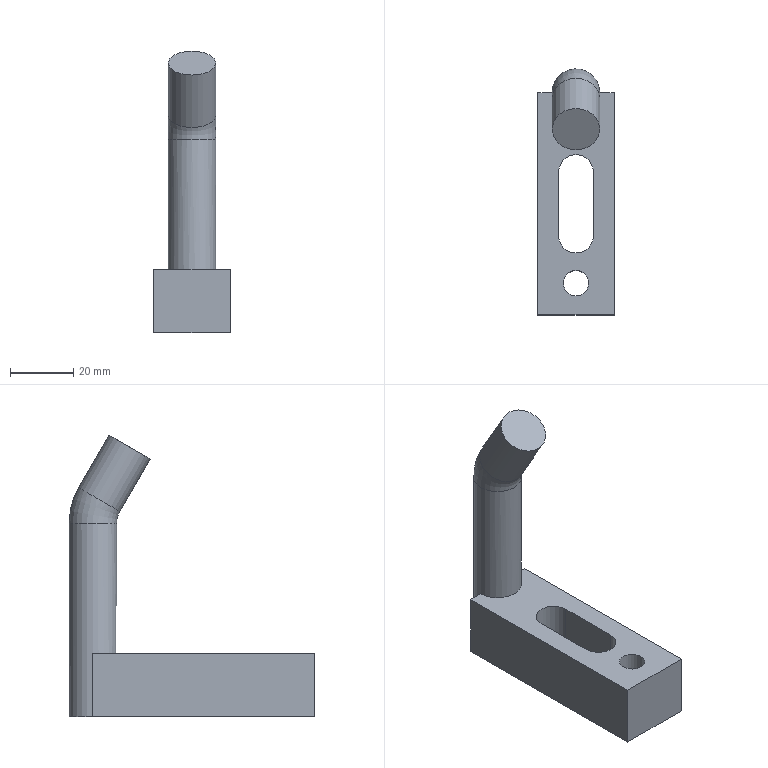Part | NX | features solid 2 | 1 solid | 16 faces | box 24 x 77.5 x 88.75 mm | volume 40062 mm3 | plane 10 | cylinder 5 | torus 1 | commonest cylinder face diameters 11 x2 15 x2 8 x1
STEP:
#1=CARTESIAN_POINT('',(67.5,315.,-15.));
#2=VERTEX_POINT('',#1);
#3=CARTESIAN_POINT('',(63.,315.,-15.));
#4=VERTEX_POINT('',#3);
#5=CARTESIAN_POINT('',(87.,315.,-15.));
#6=DIRECTION('',(-1.,0.,0.));
#7=VECTOR('',#6,1000.);
#8=LINE('',#5,#7);
#9=EDGE_CURVE('',#2,#4,#8,.T.);
#10=ORIENTED_EDGE('',*,*,#9,.F.);
#11=CARTESIAN_POINT('',(82.5,315.,-15.));
#12=VERTEX_POINT('',#11);
#13=CARTESIAN_POINT('',(75.,315.,-15.));
#14=DIRECTION('',(0.,0.,1.));
#15=DIRECTION('',(0.,-1.,0.));
#16=AXIS2_PLACEMENT_3D('',#13,#14,#15);
#17=CIRCLE('',#16,7.5);
#18=EDGE_CURVE('',#12,#2,#17,.T.);
#19=ORIENTED_EDGE('',*,*,#18,.F.);
#20=CARTESIAN_POINT('',(87.,315.,-15.));
#21=VERTEX_POINT('',#20);
#22=CARTESIAN_POINT('',(87.,315.,-15.));
#23=DIRECTION('',(-1.,0.,0.));
#24=VECTOR('',#23,1000.);
#25=LINE('',#22,#24);
#26=EDGE_CURVE('',#21,#12,#25,.T.);
#27=ORIENTED_EDGE('',*,*,#26,.F.);
#28=CARTESIAN_POINT('',(87.,245.,-15.));
#29=VERTEX_POINT('',#28);
#30=CARTESIAN_POINT('',(87.,245.,-15.));
#31=DIRECTION('',(0.,1.,0.));
#32=VECTOR('',#31,1000.);
#33=LINE('',#30,#32);
#34=EDGE_CURVE('',#29,#21,#33,.T.);
#35=ORIENTED_EDGE('',*,*,#34,.F.);
#36=CARTESIAN_POINT('',(63.,245.,-15.));
#37=VERTEX_POINT('',#36);
#38=CARTESIAN_POINT('',(63.,245.,-15.));
#39=DIRECTION('',(1.,0.,0.));
#40=VECTOR('',#39,1000.);
#41=LINE('',#38,#40);
#42=EDGE_CURVE('',#37,#29,#41,.T.);
#43=ORIENTED_EDGE('',*,*,#42,.F.);
#44=CARTESIAN_POINT('',(63.,315.,-15.));
#45=DIRECTION('',(0.,-1.,0.));
#46=VECTOR('',#45,1000.);
#47=LINE('',#44,#46);
#48=EDGE_CURVE('',#4,#37,#47,.T.);
#49=ORIENTED_EDGE('',*,*,#48,.F.);
#50=EDGE_LOOP('',(#10,#19,#27,#35,#43,#49));
#51=FACE_BOUND('',#50,.T.);
#52=CARTESIAN_POINT('',(69.5,270.,-15.));
#53=VERTEX_POINT('',#52);
#54=CARTESIAN_POINT('',(80.5,270.,-15.));
#55=VERTEX_POINT('',#54);
#56=CARTESIAN_POINT('',(75.,270.,-15.));
#57=DIRECTION('',(0.,0.,1.));
#58=DIRECTION('',(0.,-1.,0.));
#59=AXIS2_PLACEMENT_3D('',#56,#57,#58);
#60=CIRCLE('',#59,5.5);
#61=EDGE_CURVE('',#53,#55,#60,.T.);
#62=ORIENTED_EDGE('',*,*,#61,.T.);
#63=CARTESIAN_POINT('',(80.5,290.,-15.));
#64=VERTEX_POINT('',#63);
#65=CARTESIAN_POINT('',(80.5,290.,-15.));
#66=DIRECTION('',(0.,-1.,0.));
#67=VECTOR('',#66,1000.);
#68=LINE('',#65,#67);
#69=EDGE_CURVE('',#64,#55,#68,.T.);
#70=ORIENTED_EDGE('',*,*,#69,.F.);
#71=CARTESIAN_POINT('',(69.5,290.,-15.));
#72=VERTEX_POINT('',#71);
#73=CARTESIAN_POINT('',(75.,290.,-15.));
#74=DIRECTION('',(0.,0.,1.));
#75=DIRECTION('',(0.,-1.,0.));
#76=AXIS2_PLACEMENT_3D('',#73,#74,#75);
#77=CIRCLE('',#76,5.5);
#78=EDGE_CURVE('',#64,#72,#77,.T.);
#79=ORIENTED_EDGE('',*,*,#78,.T.);
#80=CARTESIAN_POINT('',(69.5,290.,-15.));
#81=DIRECTION('',(0.,-1.,0.));
#82=VECTOR('',#81,1000.);
#83=LINE('',#80,#82);
#84=EDGE_CURVE('',#72,#53,#83,.T.);
#85=ORIENTED_EDGE('',*,*,#84,.T.);
#86=EDGE_LOOP('',(#62,#70,#79,#85));
#87=FACE_BOUND('',#86,.T.);
#88=CARTESIAN_POINT('',(75.,251.,-15.));
#89=VERTEX_POINT('',#88);
#90=CARTESIAN_POINT('',(75.,255.,-15.));
#91=DIRECTION('',(0.,0.,1.));
#92=DIRECTION('',(0.,-1.,0.));
#93=AXIS2_PLACEMENT_3D('',#90,#91,#92);
#94=CIRCLE('',#93,4.);
#95=EDGE_CURVE('',#89,#89,#94,.T.);
#96=ORIENTED_EDGE('',*,*,#95,.T.);
#97=EDGE_LOOP('',(#96));
#98=FACE_BOUND('',#97,.T.);
#99=CARTESIAN_POINT('',(87.,245.,-15.));
#100=DIRECTION('',(0.,0.,1.));
#101=DIRECTION('',(0.,-1.,0.));
#102=AXIS2_PLACEMENT_3D('',#99,#100,#101);
#103=PLANE('',#102);
#104=ADVANCED_FACE('',(#51,#87,#98),#103,.F.);
#105=ORIENTED_EDGE('',*,*,#34,.T.);
#106=CARTESIAN_POINT('',(87.,315.,5.));
#107=VERTEX_POINT('',#106);
#108=CARTESIAN_POINT('',(87.,315.,5.));
#109=DIRECTION('',(0.,0.,-1.));
#110=VECTOR('',#109,1000.);
#111=LINE('',#108,#110);
#112=EDGE_CURVE('',#107,#21,#111,.T.);
#113=ORIENTED_EDGE('',*,*,#112,.F.);
#114=CARTESIAN_POINT('',(87.,245.,5.));
#115=VERTEX_POINT('',#114);
#116=CARTESIAN_POINT('',(87.,245.,5.));
#117=DIRECTION('',(0.,1.,0.));
#118=VECTOR('',#117,1000.);
#119=LINE('',#116,#118);
#120=EDGE_CURVE('',#115,#107,#119,.T.);
#121=ORIENTED_EDGE('',*,*,#120,.F.);
#122=CARTESIAN_POINT('',(87.,245.,5.));
#123=DIRECTION('',(0.,0.,-1.));
#124=VECTOR('',#123,1000.);
#125=LINE('',#122,#124);
#126=EDGE_CURVE('',#115,#29,#125,.T.);
#127=ORIENTED_EDGE('',*,*,#126,.T.);
#128=EDGE_LOOP('',(#105,#113,#121,#127));
#129=FACE_BOUND('',#128,.T.);
#130=CARTESIAN_POINT('',(87.,245.,5.));
#131=DIRECTION('',(-1.,0.,0.));
#132=DIRECTION('',(0.,-1.,0.));
#133=AXIS2_PLACEMENT_3D('',#130,#131,#132);
#134=PLANE('',#133);
#135=ADVANCED_FACE('',(#129),#134,.F.);
#136=ORIENTED_EDGE('',*,*,#42,.T.);
#137=ORIENTED_EDGE('',*,*,#126,.F.);
#138=CARTESIAN_POINT('',(63.,245.,5.));
#139=VERTEX_POINT('',#138);
#140=CARTESIAN_POINT('',(63.,245.,5.));
#141=DIRECTION('',(1.,0.,0.));
#142=VECTOR('',#141,1000.);
#143=LINE('',#140,#142);
#144=EDGE_CURVE('',#139,#115,#143,.T.);
#145=ORIENTED_EDGE('',*,*,#144,.F.);
#146=CARTESIAN_POINT('',(63.,245.,5.));
#147=DIRECTION('',(0.,0.,-1.));
#148=VECTOR('',#147,1000.);
#149=LINE('',#146,#148);
#150=EDGE_CURVE('',#139,#37,#149,.T.);
#151=ORIENTED_EDGE('',*,*,#150,.T.);
#152=EDGE_LOOP('',(#136,#137,#145,#151));
#153=FACE_BOUND('',#152,.T.);
#154=CARTESIAN_POINT('',(63.,245.,5.));
#155=DIRECTION('',(0.,1.,0.));
#156=DIRECTION('',(0.,0.,1.));
#157=AXIS2_PLACEMENT_3D('',#154,#155,#156);
#158=PLANE('',#157);
#159=ADVANCED_FACE('',(#153),#158,.F.);
#160=ORIENTED_EDGE('',*,*,#48,.T.);
#161=ORIENTED_EDGE('',*,*,#150,.F.);
#162=CARTESIAN_POINT('',(63.,315.,5.));
#163=VERTEX_POINT('',#162);
#164=CARTESIAN_POINT('',(63.,315.,5.));
#165=DIRECTION('',(0.,-1.,0.));
#166=VECTOR('',#165,1000.);
#167=LINE('',#164,#166);
#168=EDGE_CURVE('',#163,#139,#167,.T.);
#169=ORIENTED_EDGE('',*,*,#168,.F.);
#170=CARTESIAN_POINT('',(63.,315.,5.));
#171=DIRECTION('',(0.,0.,-1.));
#172=VECTOR('',#171,1000.);
#173=LINE('',#170,#172);
#174=EDGE_CURVE('',#163,#4,#173,.T.);
#175=ORIENTED_EDGE('',*,*,#174,.T.);
#176=EDGE_LOOP('',(#160,#161,#169,#175));
#177=FACE_BOUND('',#176,.T.);
#178=CARTESIAN_POINT('',(63.,315.,5.));
#179=DIRECTION('',(1.,0.,0.));
#180=DIRECTION('',(0.,1.,0.));
#181=AXIS2_PLACEMENT_3D('',#178,#179,#180);
#182=PLANE('',#181);
#183=ADVANCED_FACE('',(#177),#182,.F.);
#184=CARTESIAN_POINT('',(67.5,315.,5.));
#185=VERTEX_POINT('',#184);
#186=CARTESIAN_POINT('',(67.5,315.,40.981));
#187=DIRECTION('',(0.,0.,-1.));
#188=VECTOR('',#187,1000.);
#189=LINE('',#186,#188);
#190=EDGE_CURVE('',#2,#185,#189,.F.);
#191=ORIENTED_EDGE('',*,*,#190,.F.);
#192=ORIENTED_EDGE('',*,*,#9,.T.);
#193=ORIENTED_EDGE('',*,*,#174,.F.);
#194=CARTESIAN_POINT('',(87.,315.,5.));
#195=DIRECTION('',(-1.,0.,0.));
#196=VECTOR('',#195,1000.);
#197=LINE('',#194,#196);
#198=EDGE_CURVE('',#185,#163,#197,.T.);
#199=ORIENTED_EDGE('',*,*,#198,.F.);
#200=EDGE_LOOP('',(#191,#192,#193,#199));
#201=FACE_BOUND('',#200,.T.);
#202=CARTESIAN_POINT('',(87.,315.,5.));
#203=DIRECTION('',(0.,-1.,0.));
#204=DIRECTION('',(0.,0.,-1.));
#205=AXIS2_PLACEMENT_3D('',#202,#203,#204);
#206=PLANE('',#205);
#207=ADVANCED_FACE('',(#201),#206,.F.);
#208=ORIENTED_EDGE('',*,*,#190,.T.);
#209=CARTESIAN_POINT('',(82.5,315.,5.));
#210=VERTEX_POINT('',#209);
#211=CARTESIAN_POINT('',(75.,315.,5.));
#212=DIRECTION('',(0.,0.,1.));
#213=DIRECTION('',(1.,0.,0.));
#214=AXIS2_PLACEMENT_3D('',#211,#212,#213);
#215=CIRCLE('',#214,7.5);
#216=EDGE_CURVE('',#185,#210,#215,.T.);
#217=ORIENTED_EDGE('',*,*,#216,.T.);
#218=CARTESIAN_POINT('',(82.5,315.,40.981));
#219=DIRECTION('',(0.,0.,-1.));
#220=VECTOR('',#219,1000.);
#221=LINE('',#218,#220);
#222=EDGE_CURVE('',#210,#12,#221,.T.);
#223=ORIENTED_EDGE('',*,*,#222,.T.);
#224=ORIENTED_EDGE('',*,*,#18,.T.);
#225=EDGE_LOOP('',(#208,#217,#223,#224));
#226=FACE_BOUND('',#225,.T.);
#227=CARTESIAN_POINT('',(75.,307.5,45.981));
#228=VERTEX_POINT('',#227);
#229=CARTESIAN_POINT('',(75.,315.,45.981));
#230=DIRECTION('',(0.,0.,1.));
#231=DIRECTION('',(0.,-1.,0.));
#232=AXIS2_PLACEMENT_3D('',#229,#230,#231);
#233=CIRCLE('',#232,7.5);
#234=EDGE_CURVE('',#228,#228,#233,.T.);
#235=ORIENTED_EDGE('',*,*,#234,.F.);
#236=EDGE_LOOP('',(#235));
#237=FACE_BOUND('',#236,.T.);
#238=CARTESIAN_POINT('',(75.,315.,40.981));
#239=DIRECTION('',(0.,0.,-1.));
#240=DIRECTION('',(0.,1.,0.));
#241=AXIS2_PLACEMENT_3D('',#238,#239,#240);
#242=CYLINDRICAL_SURFACE('',#241,7.5);
#243=ADVANCED_FACE('',(#226,#237),#242,.T.);
#244=ORIENTED_EDGE('',*,*,#222,.F.);
#245=CARTESIAN_POINT('',(87.,315.,5.));
#246=DIRECTION('',(-1.,0.,0.));
#247=VECTOR('',#246,1000.);
#248=LINE('',#245,#247);
#249=EDGE_CURVE('',#107,#210,#248,.T.);
#250=ORIENTED_EDGE('',*,*,#249,.F.);
#251=ORIENTED_EDGE('',*,*,#112,.T.);
#252=ORIENTED_EDGE('',*,*,#26,.T.);
#253=EDGE_LOOP('',(#244,#250,#251,#252));
#254=FACE_BOUND('',#253,.T.);
#255=CARTESIAN_POINT('',(87.,315.,5.));
#256=DIRECTION('',(0.,-1.,0.));
#257=DIRECTION('',(0.,0.,-1.));
#258=AXIS2_PLACEMENT_3D('',#255,#256,#257);
#259=PLANE('',#258);
#260=ADVANCED_FACE('',(#254),#259,.F.);
#261=CARTESIAN_POINT('',(75.,259.,5.));
#262=VERTEX_POINT('',#261);
#263=CARTESIAN_POINT('',(75.,255.,5.));
#264=DIRECTION('',(0.,0.,-1.));
#265=DIRECTION('',(0.,1.,0.));
#266=AXIS2_PLACEMENT_3D('',#263,#264,#265);
#267=CIRCLE('',#266,4.);
#268=EDGE_CURVE('',#262,#262,#267,.T.);
#269=ORIENTED_EDGE('',*,*,#268,.F.);
#270=EDGE_LOOP('',(#269));
#271=FACE_BOUND('',#270,.T.);
#272=ORIENTED_EDGE('',*,*,#95,.F.);
#273=EDGE_LOOP('',(#272));
#274=FACE_BOUND('',#273,.T.);
#275=CARTESIAN_POINT('',(75.,255.,5.));
#276=DIRECTION('',(0.,0.,-1.));
#277=DIRECTION('',(0.,1.,0.));
#278=AXIS2_PLACEMENT_3D('',#275,#276,#277);
#279=CYLINDRICAL_SURFACE('',#278,4.);
#280=ADVANCED_FACE('',(#271,#274),#279,.F.);
#281=CARTESIAN_POINT('',(80.5,290.,5.));
#282=VERTEX_POINT('',#281);
#283=CARTESIAN_POINT('',(69.5,290.,5.));
#284=VERTEX_POINT('',#283);
#285=CARTESIAN_POINT('',(75.,290.,5.));
#286=DIRECTION('',(0.,0.,1.));
#287=DIRECTION('',(0.,-1.,0.));
#288=AXIS2_PLACEMENT_3D('',#285,#286,#287);
#289=CIRCLE('',#288,5.5);
#290=EDGE_CURVE('',#282,#284,#289,.T.);
#291=ORIENTED_EDGE('',*,*,#290,.T.);
#292=CARTESIAN_POINT('',(69.5,290.,5.));
#293=DIRECTION('',(0.,0.,1.));
#294=VECTOR('',#293,1000.);
#295=LINE('',#292,#294);
#296=EDGE_CURVE('',#72,#284,#295,.T.);
#297=ORIENTED_EDGE('',*,*,#296,.F.);
#298=ORIENTED_EDGE('',*,*,#78,.F.);
#299=CARTESIAN_POINT('',(80.5,290.,5.));
#300=DIRECTION('',(0.,0.,1.));
#301=VECTOR('',#300,1000.);
#302=LINE('',#299,#301);
#303=EDGE_CURVE('',#64,#282,#302,.T.);
#304=ORIENTED_EDGE('',*,*,#303,.T.);
#305=EDGE_LOOP('',(#291,#297,#298,#304));
#306=FACE_BOUND('',#305,.T.);
#307=CARTESIAN_POINT('',(75.,290.,5.));
#308=DIRECTION('',(0.,0.,1.));
#309=DIRECTION('',(0.,-1.,0.));
#310=AXIS2_PLACEMENT_3D('',#307,#308,#309);
#311=CYLINDRICAL_SURFACE('',#310,5.5);
#312=ADVANCED_FACE('',(#306),#311,.F.);
#313=CARTESIAN_POINT('',(69.5,270.,5.));
#314=VERTEX_POINT('',#313);
#315=CARTESIAN_POINT('',(69.5,280.,5.));
#316=DIRECTION('',(0.,-1.,0.));
#317=VECTOR('',#316,1000.);
#318=LINE('',#315,#317);
#319=EDGE_CURVE('',#284,#314,#318,.T.);
#320=ORIENTED_EDGE('',*,*,#319,.T.);
#321=CARTESIAN_POINT('',(69.5,270.,5.));
#322=DIRECTION('',(0.,0.,1.));
#323=VECTOR('',#322,1000.);
#324=LINE('',#321,#323);
#325=EDGE_CURVE('',#53,#314,#324,.T.);
#326=ORIENTED_EDGE('',*,*,#325,.F.);
#327=ORIENTED_EDGE('',*,*,#84,.F.);
#328=ORIENTED_EDGE('',*,*,#296,.T.);
#329=EDGE_LOOP('',(#320,#326,#327,#328));
#330=FACE_BOUND('',#329,.T.);
#331=CARTESIAN_POINT('',(69.5,280.,5.));
#332=DIRECTION('',(-1.,0.,0.));
#333=DIRECTION('',(0.,0.,-1.));
#334=AXIS2_PLACEMENT_3D('',#331,#332,#333);
#335=PLANE('',#334);
#336=ADVANCED_FACE('',(#330),#335,.F.);
#337=CARTESIAN_POINT('',(80.5,270.,5.));
#338=VERTEX_POINT('',#337);
#339=CARTESIAN_POINT('',(75.,270.,5.));
#340=DIRECTION('',(0.,0.,1.));
#341=DIRECTION('',(0.,-1.,0.));
#342=AXIS2_PLACEMENT_3D('',#339,#340,#341);
#343=CIRCLE('',#342,5.5);
#344=EDGE_CURVE('',#314,#338,#343,.T.);
#345=ORIENTED_EDGE('',*,*,#344,.T.);
#346=CARTESIAN_POINT('',(80.5,270.,5.));
#347=DIRECTION('',(0.,0.,1.));
#348=VECTOR('',#347,1000.);
#349=LINE('',#346,#348);
#350=EDGE_CURVE('',#55,#338,#349,.T.);
#351=ORIENTED_EDGE('',*,*,#350,.F.);
#352=ORIENTED_EDGE('',*,*,#61,.F.);
#353=ORIENTED_EDGE('',*,*,#325,.T.);
#354=EDGE_LOOP('',(#345,#351,#352,#353));
#355=FACE_BOUND('',#354,.T.);
#356=CARTESIAN_POINT('',(75.,270.,5.));
#357=DIRECTION('',(0.,0.,1.));
#358=DIRECTION('',(0.,-1.,0.));
#359=AXIS2_PLACEMENT_3D('',#356,#357,#358);
#360=CYLINDRICAL_SURFACE('',#359,5.5);
#361=ADVANCED_FACE('',(#355),#360,.F.);
#362=CARTESIAN_POINT('',(80.5,280.,5.));
#363=DIRECTION('',(0.,-1.,0.));
#364=VECTOR('',#363,1000.);
#365=LINE('',#362,#364);
#366=EDGE_CURVE('',#282,#338,#365,.T.);
#367=ORIENTED_EDGE('',*,*,#366,.F.);
#368=ORIENTED_EDGE('',*,*,#303,.F.);
#369=ORIENTED_EDGE('',*,*,#69,.T.);
#370=ORIENTED_EDGE('',*,*,#350,.T.);
#371=EDGE_LOOP('',(#367,#368,#369,#370));
#372=FACE_BOUND('',#371,.T.);
#373=CARTESIAN_POINT('',(80.5,280.,5.));
#374=DIRECTION('',(1.,0.,0.));
#375=DIRECTION('',(0.,0.,1.));
#376=AXIS2_PLACEMENT_3D('',#373,#374,#375);
#377=PLANE('',#376);
#378=ADVANCED_FACE('',(#372),#377,.F.);
#379=ORIENTED_EDGE('',*,*,#216,.F.);
#380=ORIENTED_EDGE('',*,*,#198,.T.);
#381=ORIENTED_EDGE('',*,*,#168,.T.);
#382=ORIENTED_EDGE('',*,*,#144,.T.);
#383=ORIENTED_EDGE('',*,*,#120,.T.);
#384=ORIENTED_EDGE('',*,*,#249,.T.);
#385=EDGE_LOOP('',(#379,#380,#381,#382,#383,#384));
#386=FACE_BOUND('',#385,.T.);
#387=ORIENTED_EDGE('',*,*,#366,.T.);
#388=ORIENTED_EDGE('',*,*,#344,.F.);
#389=ORIENTED_EDGE('',*,*,#319,.F.);
#390=ORIENTED_EDGE('',*,*,#290,.F.);
#391=EDGE_LOOP('',(#387,#388,#389,#390));
#392=FACE_BOUND('',#391,.T.);
#393=ORIENTED_EDGE('',*,*,#268,.T.);
#394=EDGE_LOOP('',(#393));
#395=FACE_BOUND('',#394,.T.);
#396=CARTESIAN_POINT('',(87.,245.,5.));
#397=DIRECTION('',(0.,0.,1.));
#398=DIRECTION('',(0.,-1.,0.));
#399=AXIS2_PLACEMENT_3D('',#396,#397,#398);
#400=PLANE('',#399);
#401=ADVANCED_FACE('',(#386,#392,#395),#400,.T.);
#402=CARTESIAN_POINT('',(75.,306.495,49.731));
#403=VERTEX_POINT('',#402);
#404=CARTESIAN_POINT('',(75.,312.99,53.481));
#405=DIRECTION('',(0.,-0.5,0.866));
#406=DIRECTION('',(0.,-0.866,-0.5));
#407=AXIS2_PLACEMENT_3D('',#404,#405,#406);
#408=CIRCLE('',#407,7.5);
#409=EDGE_CURVE('',#403,#403,#408,.T.);
#410=ORIENTED_EDGE('',*,*,#409,.T.);
#411=EDGE_LOOP('',(#410));
#412=FACE_BOUND('',#411,.T.);
#413=CARTESIAN_POINT('',(75.,296.958,66.25));
#414=VERTEX_POINT('',#413);
#415=CARTESIAN_POINT('',(75.,303.453,70.));
#416=DIRECTION('',(0.,-0.5,0.866));
#417=DIRECTION('',(0.,-0.866,-0.5));
#418=AXIS2_PLACEMENT_3D('',#415,#416,#417);
#419=CIRCLE('',#418,7.5);
#420=EDGE_CURVE('',#414,#414,#419,.T.);
#421=ORIENTED_EDGE('',*,*,#420,.F.);
#422=EDGE_LOOP('',(#421));
#423=FACE_BOUND('',#422,.T.);
#424=CARTESIAN_POINT('',(75.,312.99,53.481));
#425=DIRECTION('',(0.,-0.5,0.866));
#426=DIRECTION('',(0.,-0.866,-0.5));
#427=AXIS2_PLACEMENT_3D('',#424,#425,#426);
#428=CYLINDRICAL_SURFACE('',#427,7.5);
#429=ADVANCED_FACE('',(#412,#423),#428,.T.);
#430=ORIENTED_EDGE('',*,*,#234,.T.);
#431=EDGE_LOOP('',(#430));
#432=FACE_BOUND('',#431,.T.);
#433=ORIENTED_EDGE('',*,*,#409,.F.);
#434=EDGE_LOOP('',(#433));
#435=FACE_BOUND('',#434,.T.);
#436=CARTESIAN_POINT('',(75.,300.,45.981));
#437=DIRECTION('',(1.,0.,0.));
#438=DIRECTION('',(0.,0.,1.));
#439=AXIS2_PLACEMENT_3D('',#436,#437,#438);
#440=TOROIDAL_SURFACE('',#439,15.,7.5);
#441=ADVANCED_FACE('',(#432,#435),#440,.T.);
#442=ORIENTED_EDGE('',*,*,#420,.T.);
#443=EDGE_LOOP('',(#442));
#444=FACE_BOUND('',#443,.T.);
#445=CARTESIAN_POINT('',(75.,303.453,70.));
#446=DIRECTION('',(0.,-0.5,0.866));
#447=DIRECTION('',(0.,-0.866,-0.5));
#448=AXIS2_PLACEMENT_3D('',#445,#446,#447);
#449=PLANE('',#448);
#450=ADVANCED_FACE('',(#444),#449,.T.);
#451=CLOSED_SHELL('',(#104,#135,#159,#183,#207,#243,#260,#280,#312,#336,#361,#378,#401,#429,#441,#450));
#452=MANIFOLD_SOLID_BREP('',#451);
#453=(LENGTH_UNIT()NAMED_UNIT(*)SI_UNIT(.MILLI.,.METRE.));
#454=UNCERTAINTY_MEASURE_WITH_UNIT(LENGTH_MEASURE(0.00001),#453,'','');
#455=(NAMED_UNIT(*)PLANE_ANGLE_UNIT()SI_UNIT($,.RADIAN.));
#456=(NAMED_UNIT(*)SI_UNIT($,.STERADIAN.)SOLID_ANGLE_UNIT());
#457=(GEOMETRIC_REPRESENTATION_CONTEXT(3)GLOBAL_UNCERTAINTY_ASSIGNED_CONTEXT((#454))GLOBAL_UNIT_ASSIGNED_CONTEXT((#453,#455,#456))REPRESENTATION_CONTEXT('',''));
#458=ADVANCED_BREP_SHAPE_REPRESENTATION('',(#452),#457);